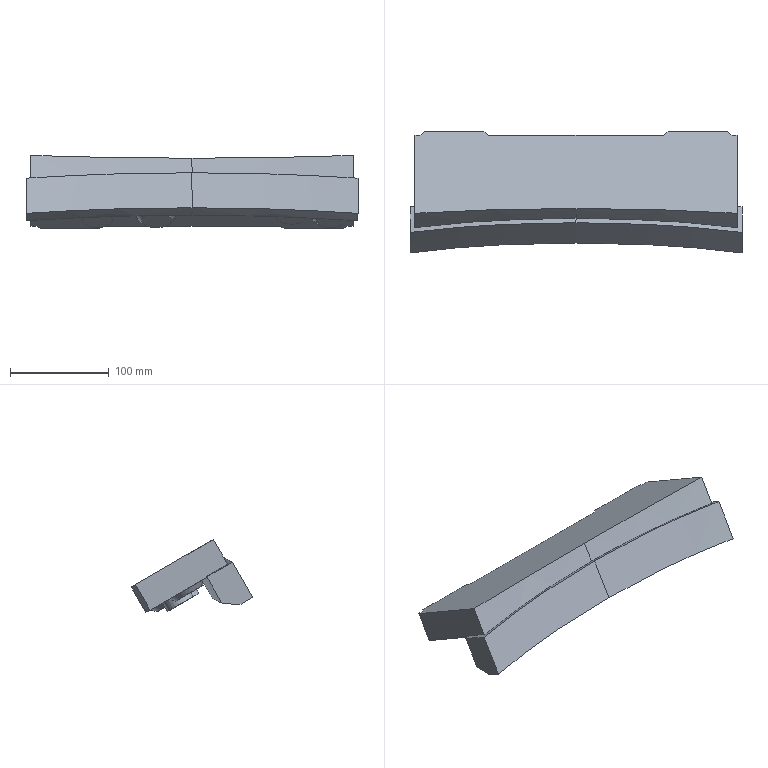Part | NX | features solid 2 | 1 solid | 39 faces | box 336.667 x 123.505 x 74.124 mm | volume 1242593 mm3 | plane 21 | spline 12 | cone 4 | cylinder 2 | commonest cylinder face diameters 30 x2